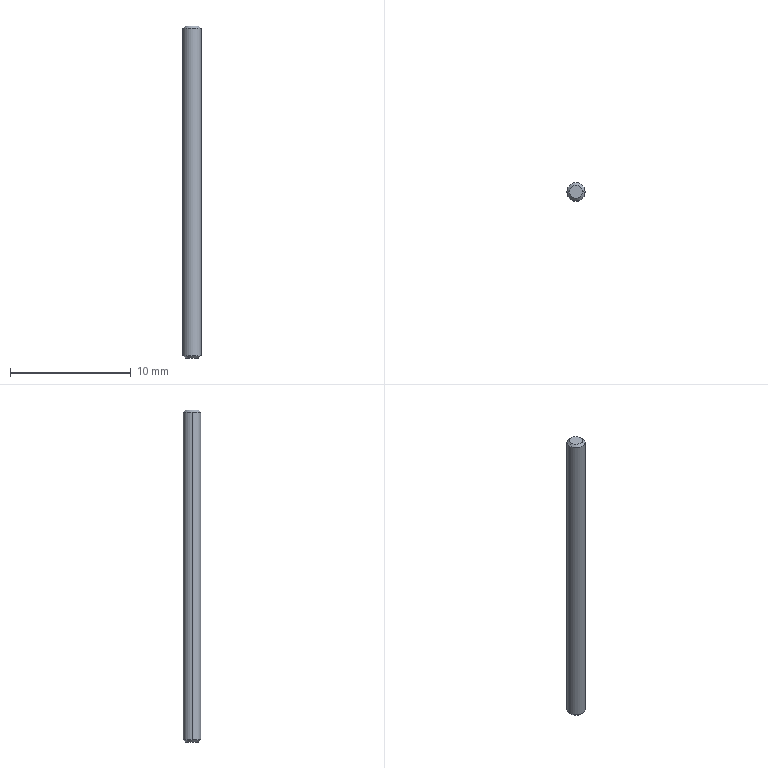Part | SolidWorks | features Chamfer 1, Extrusion 1 | 1 solid | 8 faces | box 1.5 x 1.5 x 27.5 mm | volume 48.425 mm3 | cone 4 | cylinder 2 | plane 2 | commonest cylinder face diameters 1.5 x2
STEP:
#1=CARTESIAN_POINT('',(0.55,0.,13.75));
#2=VERTEX_POINT('',#1);
#3=CARTESIAN_POINT('',(-0.55,0.,13.75));
#4=VERTEX_POINT('',#3);
#5=CARTESIAN_POINT('',(0.,0.,13.75));
#6=DIRECTION('',(0.,0.,1.));
#7=DIRECTION('',(1.,0.,0.));
#8=AXIS2_PLACEMENT_3D('',#5,#6,#7);
#9=CIRCLE('',#8,0.55);
#10=EDGE_CURVE('',#2,#4,#9,.T.);
#11=ORIENTED_EDGE('',*,*,#10,.F.);
#12=CARTESIAN_POINT('',(0.75,0.,13.55));
#13=VERTEX_POINT('',#12);
#14=CARTESIAN_POINT('',(0.55,0.,13.75));
#15=DIRECTION('',(0.7071,0.,-0.7071));
#16=VECTOR('',#15,1000.);
#17=LINE('',#14,#16);
#18=EDGE_CURVE('',#2,#13,#17,.T.);
#19=ORIENTED_EDGE('',*,*,#18,.T.);
#20=CARTESIAN_POINT('',(-0.75,0.,13.55));
#21=VERTEX_POINT('',#20);
#22=CARTESIAN_POINT('',(0.,0.,13.55));
#23=DIRECTION('',(0.,0.,-1.));
#24=DIRECTION('',(1.,0.,0.));
#25=AXIS2_PLACEMENT_3D('',#22,#23,#24);
#26=CIRCLE('',#25,0.75);
#27=EDGE_CURVE('',#21,#13,#26,.T.);
#28=ORIENTED_EDGE('',*,*,#27,.F.);
#29=CARTESIAN_POINT('',(-0.55,0.,13.75));
#30=DIRECTION('',(-0.7071,0.,-0.7071));
#31=VECTOR('',#30,1000.);
#32=LINE('',#29,#31);
#33=EDGE_CURVE('',#4,#21,#32,.T.);
#34=ORIENTED_EDGE('',*,*,#33,.F.);
#35=EDGE_LOOP('',(#11,#19,#28,#34));
#36=FACE_OUTER_BOUND('',#35,.T.);
#37=CARTESIAN_POINT('',(0.,0.,13.75));
#38=DIRECTION('',(0.,0.,-1.));
#39=DIRECTION('',(-1.,0.,0.));
#40=AXIS2_PLACEMENT_3D('',#37,#38,#39);
#41=CONICAL_SURFACE('',#40,0.55,0.7854);
#42=ADVANCED_FACE('',(#36),#41,.T.);
#43=CARTESIAN_POINT('',(-0.55,0.,-13.75));
#44=VERTEX_POINT('',#43);
#45=CARTESIAN_POINT('',(0.55,0.,-13.75));
#46=VERTEX_POINT('',#45);
#47=CARTESIAN_POINT('',(0.,0.,-13.75));
#48=DIRECTION('',(0.,0.,-1.));
#49=DIRECTION('',(1.,0.,0.));
#50=AXIS2_PLACEMENT_3D('',#47,#48,#49);
#51=CIRCLE('',#50,0.55);
#52=EDGE_CURVE('',#44,#46,#51,.T.);
#53=ORIENTED_EDGE('',*,*,#52,.F.);
#54=CARTESIAN_POINT('',(-0.75,0.,-13.55));
#55=VERTEX_POINT('',#54);
#56=CARTESIAN_POINT('',(-0.75,0.,-13.55));
#57=DIRECTION('',(-0.7071,0.,0.7071));
#58=VECTOR('',#57,1000.);
#59=LINE('',#56,#58);
#60=EDGE_CURVE('',#44,#55,#59,.T.);
#61=ORIENTED_EDGE('',*,*,#60,.T.);
#62=CARTESIAN_POINT('',(0.75,0.,-13.55));
#63=VERTEX_POINT('',#62);
#64=CARTESIAN_POINT('',(0.,0.,-13.55));
#65=DIRECTION('',(0.,0.,1.));
#66=DIRECTION('',(1.,0.,0.));
#67=AXIS2_PLACEMENT_3D('',#64,#65,#66);
#68=CIRCLE('',#67,0.75);
#69=EDGE_CURVE('',#63,#55,#68,.T.);
#70=ORIENTED_EDGE('',*,*,#69,.F.);
#71=CARTESIAN_POINT('',(0.75,0.,-13.55));
#72=DIRECTION('',(0.7071,0.,0.7071));
#73=VECTOR('',#72,1000.);
#74=LINE('',#71,#73);
#75=EDGE_CURVE('',#46,#63,#74,.T.);
#76=ORIENTED_EDGE('',*,*,#75,.F.);
#77=EDGE_LOOP('',(#53,#61,#70,#76));
#78=FACE_OUTER_BOUND('',#77,.T.);
#79=CARTESIAN_POINT('',(0.,0.,-13.55));
#80=DIRECTION('',(0.,0.,1.));
#81=DIRECTION('',(1.,0.,0.));
#82=AXIS2_PLACEMENT_3D('',#79,#80,#81);
#83=CONICAL_SURFACE('',#82,0.75,0.7854);
#84=ADVANCED_FACE('',(#78),#83,.T.);
#85=ORIENTED_EDGE('',*,*,#27,.T.);
#86=CARTESIAN_POINT('',(0.75,0.,13.75));
#87=DIRECTION('',(0.,0.,-1.));
#88=VECTOR('',#87,1000.);
#89=LINE('',#86,#88);
#90=EDGE_CURVE('',#13,#63,#89,.T.);
#91=ORIENTED_EDGE('',*,*,#90,.T.);
#92=ORIENTED_EDGE('',*,*,#69,.T.);
#93=CARTESIAN_POINT('',(-0.75,0.,13.75));
#94=DIRECTION('',(0.,0.,-1.));
#95=VECTOR('',#94,1000.);
#96=LINE('',#93,#95);
#97=EDGE_CURVE('',#21,#55,#96,.T.);
#98=ORIENTED_EDGE('',*,*,#97,.F.);
#99=EDGE_LOOP('',(#85,#91,#92,#98));
#100=FACE_OUTER_BOUND('',#99,.T.);
#101=CARTESIAN_POINT('',(0.,0.,13.75));
#102=DIRECTION('',(0.,0.,-1.));
#103=DIRECTION('',(-1.,0.,0.));
#104=AXIS2_PLACEMENT_3D('',#101,#102,#103);
#105=CYLINDRICAL_SURFACE('',#104,0.75);
#106=ADVANCED_FACE('',(#100),#105,.T.);
#107=ORIENTED_EDGE('',*,*,#90,.F.);
#108=CARTESIAN_POINT('',(0.,0.,13.55));
#109=DIRECTION('',(0.,0.,-1.));
#110=DIRECTION('',(1.,0.,0.));
#111=AXIS2_PLACEMENT_3D('',#108,#109,#110);
#112=CIRCLE('',#111,0.75);
#113=EDGE_CURVE('',#13,#21,#112,.T.);
#114=ORIENTED_EDGE('',*,*,#113,.T.);
#115=ORIENTED_EDGE('',*,*,#97,.T.);
#116=CARTESIAN_POINT('',(0.,0.,-13.55));
#117=DIRECTION('',(0.,0.,1.));
#118=DIRECTION('',(1.,0.,0.));
#119=AXIS2_PLACEMENT_3D('',#116,#117,#118);
#120=CIRCLE('',#119,0.75);
#121=EDGE_CURVE('',#55,#63,#120,.T.);
#122=ORIENTED_EDGE('',*,*,#121,.T.);
#123=EDGE_LOOP('',(#107,#114,#115,#122));
#124=FACE_OUTER_BOUND('',#123,.T.);
#125=CARTESIAN_POINT('',(0.,0.,13.75));
#126=DIRECTION('',(0.,0.,-1.));
#127=DIRECTION('',(-1.,0.,0.));
#128=AXIS2_PLACEMENT_3D('',#125,#126,#127);
#129=CYLINDRICAL_SURFACE('',#128,0.75);
#130=ADVANCED_FACE('',(#124),#129,.T.);
#131=CARTESIAN_POINT('',(0.,0.,13.75));
#132=DIRECTION('',(0.,0.,1.));
#133=DIRECTION('',(1.,0.,0.));
#134=AXIS2_PLACEMENT_3D('',#131,#132,#133);
#135=CIRCLE('',#134,0.55);
#136=EDGE_CURVE('',#4,#2,#135,.T.);
#137=ORIENTED_EDGE('',*,*,#136,.T.);
#138=ORIENTED_EDGE('',*,*,#10,.T.);
#139=EDGE_LOOP('',(#137,#138));
#140=FACE_OUTER_BOUND('',#139,.T.);
#141=CARTESIAN_POINT('',(0.,0.,13.75));
#142=DIRECTION('',(0.,0.,1.));
#143=DIRECTION('',(1.,0.,0.));
#144=AXIS2_PLACEMENT_3D('',#141,#142,#143);
#145=PLANE('',#144);
#146=ADVANCED_FACE('',(#140),#145,.T.);
#147=CARTESIAN_POINT('',(0.,0.,-13.75));
#148=DIRECTION('',(0.,0.,-1.));
#149=DIRECTION('',(1.,0.,0.));
#150=AXIS2_PLACEMENT_3D('',#147,#148,#149);
#151=CIRCLE('',#150,0.55);
#152=EDGE_CURVE('',#46,#44,#151,.T.);
#153=ORIENTED_EDGE('',*,*,#152,.T.);
#154=ORIENTED_EDGE('',*,*,#52,.T.);
#155=EDGE_LOOP('',(#153,#154));
#156=FACE_OUTER_BOUND('',#155,.T.);
#157=CARTESIAN_POINT('',(0.,0.,-13.75));
#158=DIRECTION('',(0.,0.,1.));
#159=DIRECTION('',(1.,0.,0.));
#160=AXIS2_PLACEMENT_3D('',#157,#158,#159);
#161=PLANE('',#160);
#162=ADVANCED_FACE('',(#156),#161,.F.);
#163=ORIENTED_EDGE('',*,*,#60,.F.);
#164=ORIENTED_EDGE('',*,*,#152,.F.);
#165=ORIENTED_EDGE('',*,*,#75,.T.);
#166=ORIENTED_EDGE('',*,*,#121,.F.);
#167=EDGE_LOOP('',(#163,#164,#165,#166));
#168=FACE_OUTER_BOUND('',#167,.T.);
#169=CARTESIAN_POINT('',(0.,0.,-13.55));
#170=DIRECTION('',(0.,0.,1.));
#171=DIRECTION('',(1.,0.,0.));
#172=AXIS2_PLACEMENT_3D('',#169,#170,#171);
#173=CONICAL_SURFACE('',#172,0.75,0.7854);
#174=ADVANCED_FACE('',(#168),#173,.T.);
#175=ORIENTED_EDGE('',*,*,#18,.F.);
#176=ORIENTED_EDGE('',*,*,#136,.F.);
#177=ORIENTED_EDGE('',*,*,#33,.T.);
#178=ORIENTED_EDGE('',*,*,#113,.F.);
#179=EDGE_LOOP('',(#175,#176,#177,#178));
#180=FACE_OUTER_BOUND('',#179,.T.);
#181=CARTESIAN_POINT('',(0.,0.,13.75));
#182=DIRECTION('',(0.,0.,-1.));
#183=DIRECTION('',(-1.,0.,0.));
#184=AXIS2_PLACEMENT_3D('',#181,#182,#183);
#185=CONICAL_SURFACE('',#184,0.55,0.7854);
#186=ADVANCED_FACE('',(#180),#185,.T.);
#187=CLOSED_SHELL('',(#42,#84,#106,#130,#146,#162,#174,#186));
#188=MANIFOLD_SOLID_BREP('',#187);
#189=CARTESIAN_POINT('',(0.,0.,0.));
#190=DIRECTION('',(0.,0.,1.));
#191=DIRECTION('',(1.,0.,0.));
#192=AXIS2_PLACEMENT_3D('',#189,#190,#191);
#193=(LENGTH_UNIT()NAMED_UNIT(*)SI_UNIT(.MILLI.,.METRE.));
#194=UNCERTAINTY_MEASURE_WITH_UNIT(LENGTH_MEASURE(0.00001),#193,'','');
#195=(NAMED_UNIT(*)PLANE_ANGLE_UNIT()SI_UNIT($,.RADIAN.));
#196=(NAMED_UNIT(*)SI_UNIT($,.STERADIAN.)SOLID_ANGLE_UNIT());
#197=(GEOMETRIC_REPRESENTATION_CONTEXT(3)GLOBAL_UNCERTAINTY_ASSIGNED_CONTEXT((#194))GLOBAL_UNIT_ASSIGNED_CONTEXT((#193,#195,#196))REPRESENTATION_CONTEXT('',''));
#198=ADVANCED_BREP_SHAPE_REPRESENTATION('',(#188,#192),#197);